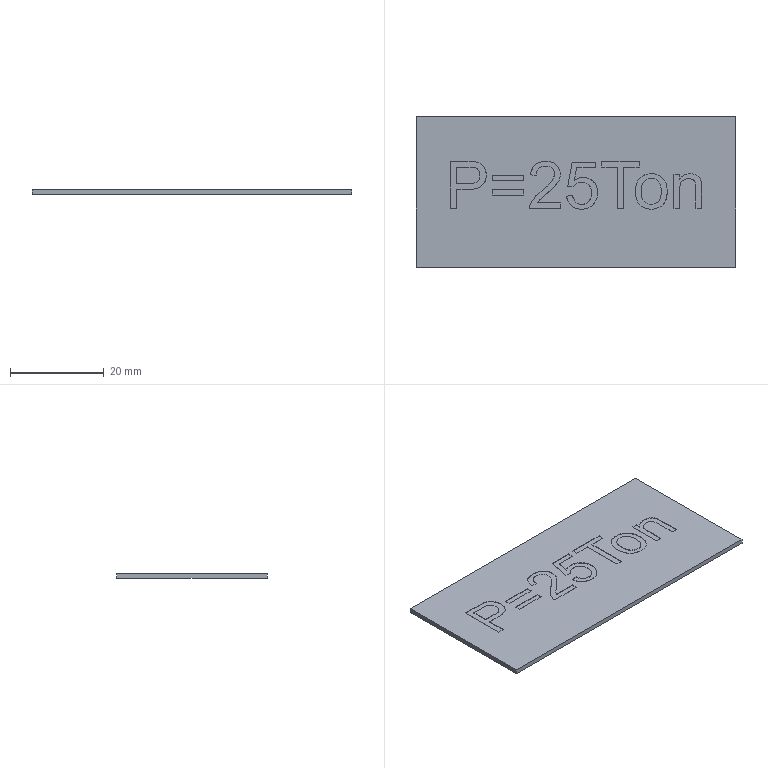Part | STEP file | lll_id958_x_t | 1 solid | 69 faces | box 68.033 x 31.95 x 1 mm | volume 2157 mm3 | plane 52 | other 17